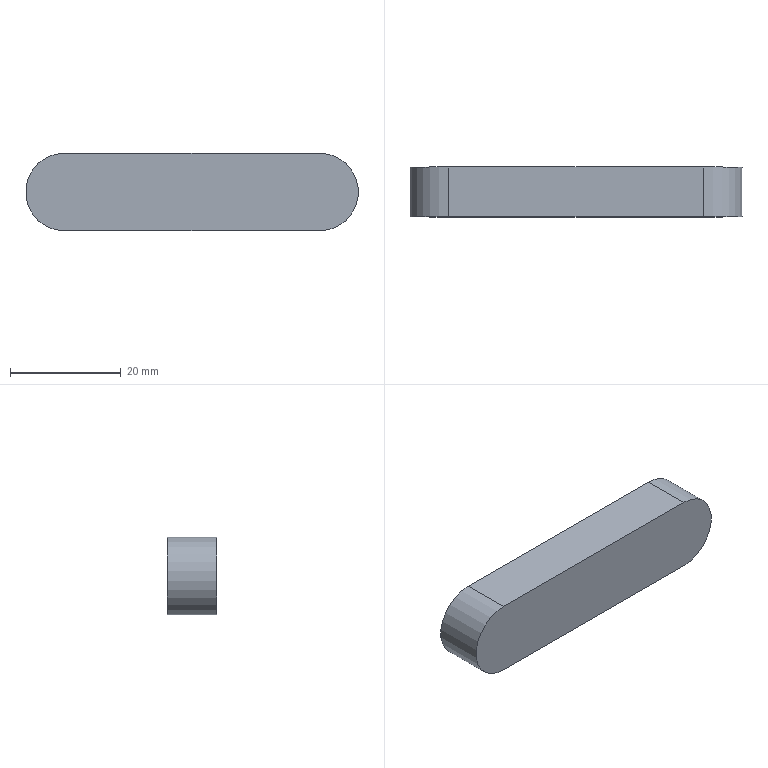Part | SolidWorks | features Extrusion 1, ICE 1 | 1 solid | 626 faces | box 60 x 9 x 14 mm | volume 7180 mm3 | plane 436 | spline 188 | cylinder 2 | commonest cylinder face diameters 14 x2